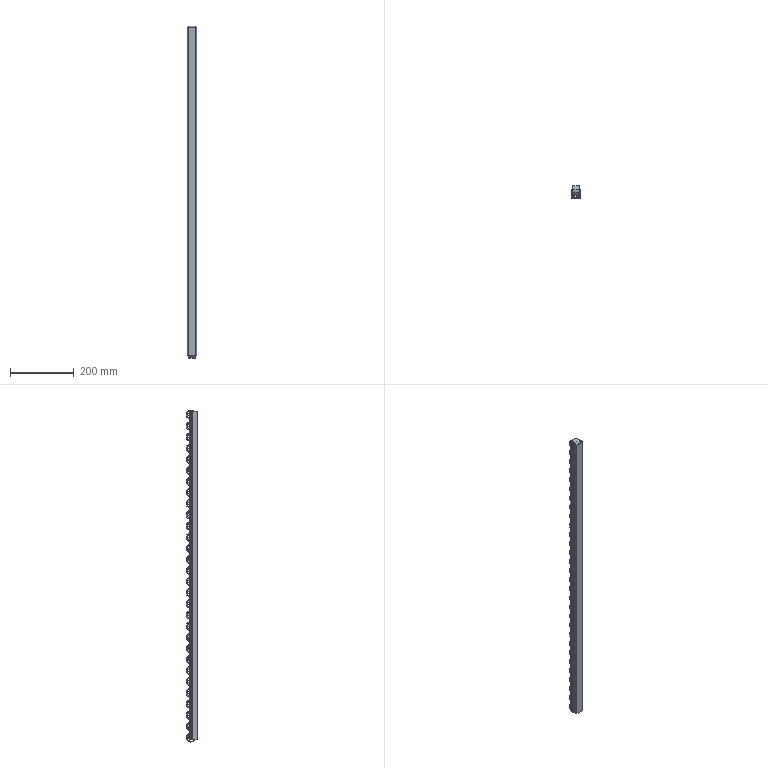Part | STEP file | RIEL FINAL NLV 3 | 40 solids | 1326 faces | box 28.4 x 36.2 x 1045 mm | volume 307295 mm3 | cylinder 674 | plane 580 | spline 72 | commonest cylinder face diameters 10 x240 25 x240 5 x60 30 x60 4 x58 1.473 x8